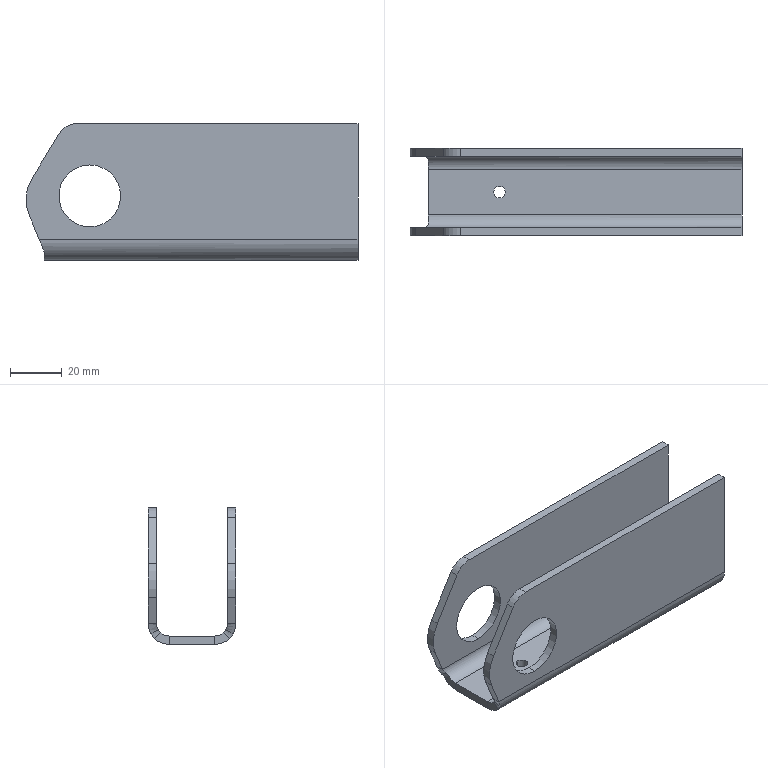Part | SolidWorks | features ICE 2, Fillet 1, FlatPattern 1, SMBaseFlange 1, SheetMetal 1 | 1 solid | 38 faces | box 128.757 x 34 x 53 mm | volume 47449 mm3 | plane 20 | cylinder 14 | spline 4 | commonest cylinder face diameters 24 x4 4.5 x2 10 x2 16 x2 16.4 x2 30 x2
STEP:
#1=CARTESIAN_POINT('',(41.,-14.75,-49.8));
#2=VERTEX_POINT('',#1);
#3=CARTESIAN_POINT('',(41.,-19.25,-49.8));
#4=VERTEX_POINT('',#3);
#5=CARTESIAN_POINT('',(41.,-17.,-49.8));
#6=DIRECTION('',(0.,0.,1.));
#7=DIRECTION('',(0.,1.,0.));
#8=AXIS2_PLACEMENT_3D('',#5,#6,#7);
#9=CIRCLE('',#8,2.25);
#10=EDGE_CURVE('',#2,#4,#9,.T.);
#11=ORIENTED_EDGE('',*,*,#10,.T.);
#12=CARTESIAN_POINT('',(41.,-19.25,-53.));
#13=VERTEX_POINT('',#12);
#14=CARTESIAN_POINT('',(41.,-19.25,0.001));
#15=DIRECTION('',(0.,0.,-1.));
#16=VECTOR('',#15,1000.);
#17=LINE('',#14,#16);
#18=EDGE_CURVE('',#4,#13,#17,.T.);
#19=ORIENTED_EDGE('',*,*,#18,.T.);
#20=CARTESIAN_POINT('',(41.,-14.75,-53.));
#21=VERTEX_POINT('',#20);
#22=CARTESIAN_POINT('',(41.,-17.,-53.));
#23=DIRECTION('',(0.,0.,-1.));
#24=DIRECTION('',(0.,1.,0.));
#25=AXIS2_PLACEMENT_3D('',#22,#23,#24);
#26=CIRCLE('',#25,2.25);
#27=EDGE_CURVE('',#13,#21,#26,.T.);
#28=ORIENTED_EDGE('',*,*,#27,.T.);
#29=CARTESIAN_POINT('',(41.,-14.75,0.001));
#30=DIRECTION('',(0.,0.,-1.));
#31=VECTOR('',#30,1000.);
#32=LINE('',#29,#31);
#33=EDGE_CURVE('',#2,#21,#32,.T.);
#34=ORIENTED_EDGE('',*,*,#33,.F.);
#35=EDGE_LOOP('',(#11,#19,#28,#34));
#36=FACE_OUTER_BOUND('',#35,.T.);
#37=CARTESIAN_POINT('',(41.,-17.,0.001));
#38=DIRECTION('',(0.,0.,-1.));
#39=DIRECTION('',(0.,1.,0.));
#40=AXIS2_PLACEMENT_3D('',#37,#38,#39);
#41=CYLINDRICAL_SURFACE('',#40,2.25);
#42=ADVANCED_FACE('',(#36),#41,.F.);
#43=CARTESIAN_POINT('',(31.,-30.8,-16.));
#44=VERTEX_POINT('',#43);
#45=CARTESIAN_POINT('',(31.,-30.8,-40.));
#46=VERTEX_POINT('',#45);
#47=CARTESIAN_POINT('',(31.,-30.8,-28.));
#48=DIRECTION('',(0.,-1.,0.));
#49=DIRECTION('',(0.,0.,1.));
#50=AXIS2_PLACEMENT_3D('',#47,#48,#49);
#51=CIRCLE('',#50,12.);
#52=EDGE_CURVE('',#44,#46,#51,.T.);
#53=ORIENTED_EDGE('',*,*,#52,.F.);
#54=CARTESIAN_POINT('',(31.,-34.,-16.));
#55=VERTEX_POINT('',#54);
#56=CARTESIAN_POINT('',(31.,-30.8,-16.));
#57=DIRECTION('',(0.,-1.,0.));
#58=VECTOR('',#57,1000.);
#59=LINE('',#56,#58);
#60=EDGE_CURVE('',#44,#55,#59,.T.);
#61=ORIENTED_EDGE('',*,*,#60,.T.);
#62=CARTESIAN_POINT('',(31.,-34.,-40.));
#63=VERTEX_POINT('',#62);
#64=CARTESIAN_POINT('',(31.,-34.,-28.));
#65=DIRECTION('',(0.,-1.,0.));
#66=DIRECTION('',(0.,0.,-1.));
#67=AXIS2_PLACEMENT_3D('',#64,#65,#66);
#68=CIRCLE('',#67,12.);
#69=EDGE_CURVE('',#55,#63,#68,.T.);
#70=ORIENTED_EDGE('',*,*,#69,.T.);
#71=CARTESIAN_POINT('',(31.,-30.8,-40.));
#72=DIRECTION('',(0.,-1.,0.));
#73=VECTOR('',#72,1000.);
#74=LINE('',#71,#73);
#75=EDGE_CURVE('',#46,#63,#74,.T.);
#76=ORIENTED_EDGE('',*,*,#75,.F.);
#77=EDGE_LOOP('',(#53,#61,#70,#76));
#78=FACE_OUTER_BOUND('',#77,.T.);
#79=CARTESIAN_POINT('',(31.,-30.8,-28.));
#80=DIRECTION('',(0.,-1.,0.));
#81=DIRECTION('',(0.,0.,-1.));
#82=AXIS2_PLACEMENT_3D('',#79,#80,#81);
#83=CYLINDRICAL_SURFACE('',#82,12.);
#84=ADVANCED_FACE('',(#78),#83,.F.);
#85=CARTESIAN_POINT('',(31.,-3.2,-40.));
#86=VERTEX_POINT('',#85);
#87=CARTESIAN_POINT('',(31.,-3.2,-16.));
#88=VERTEX_POINT('',#87);
#89=CARTESIAN_POINT('',(31.,-3.2,-28.));
#90=DIRECTION('',(0.,1.,0.));
#91=DIRECTION('',(0.,0.,-1.));
#92=AXIS2_PLACEMENT_3D('',#89,#90,#91);
#93=CIRCLE('',#92,12.);
#94=EDGE_CURVE('',#86,#88,#93,.T.);
#95=ORIENTED_EDGE('',*,*,#94,.F.);
#96=CARTESIAN_POINT('',(31.,0.,-40.));
#97=VERTEX_POINT('',#96);
#98=CARTESIAN_POINT('',(31.,-3.2,-40.));
#99=DIRECTION('',(0.,1.,0.));
#100=VECTOR('',#99,1000.);
#101=LINE('',#98,#100);
#102=EDGE_CURVE('',#86,#97,#101,.T.);
#103=ORIENTED_EDGE('',*,*,#102,.T.);
#104=CARTESIAN_POINT('',(31.,0.,-16.));
#105=VERTEX_POINT('',#104);
#106=CARTESIAN_POINT('',(31.,0.,-28.));
#107=DIRECTION('',(0.,1.,0.));
#108=DIRECTION('',(0.,0.,1.));
#109=AXIS2_PLACEMENT_3D('',#106,#107,#108);
#110=CIRCLE('',#109,12.);
#111=EDGE_CURVE('',#97,#105,#110,.T.);
#112=ORIENTED_EDGE('',*,*,#111,.T.);
#113=CARTESIAN_POINT('',(31.,-3.2,-16.));
#114=DIRECTION('',(0.,1.,0.));
#115=VECTOR('',#114,1000.);
#116=LINE('',#113,#115);
#117=EDGE_CURVE('',#88,#105,#116,.T.);
#118=ORIENTED_EDGE('',*,*,#117,.F.);
#119=EDGE_LOOP('',(#95,#103,#112,#118));
#120=FACE_OUTER_BOUND('',#119,.T.);
#121=CARTESIAN_POINT('',(31.,-3.2,-28.));
#122=DIRECTION('',(0.,1.,0.));
#123=DIRECTION('',(0.,0.,1.));
#124=AXIS2_PLACEMENT_3D('',#121,#122,#123);
#125=CYLINDRICAL_SURFACE('',#124,12.);
#126=ADVANCED_FACE('',(#120),#125,.F.);
#127=CARTESIAN_POINT('',(135.,-30.8,0.));
#128=VERTEX_POINT('',#127);
#129=CARTESIAN_POINT('',(26.002,-30.8,0.));
#130=VERTEX_POINT('',#129);
#131=CARTESIAN_POINT('',(135.,-30.8,0.));
#132=DIRECTION('',(-1.,0.,0.));
#133=VECTOR('',#132,1000.);
#134=LINE('',#131,#133);
#135=EDGE_CURVE('',#128,#130,#134,.T.);
#136=ORIENTED_EDGE('',*,*,#135,.T.);
#137=CARTESIAN_POINT('',(26.002,-34.,0.));
#138=VERTEX_POINT('',#137);
#139=CARTESIAN_POINT('',(26.002,-34.,0.));
#140=DIRECTION('',(0.,-1.,0.));
#141=VECTOR('',#140,1000.);
#142=LINE('',#139,#141);
#143=EDGE_CURVE('',#130,#138,#142,.T.);
#144=ORIENTED_EDGE('',*,*,#143,.T.);
#145=CARTESIAN_POINT('',(135.,-34.,0.));
#146=VERTEX_POINT('',#145);
#147=CARTESIAN_POINT('',(135.,-34.,0.));
#148=DIRECTION('',(-1.,0.,0.));
#149=VECTOR('',#148,1000.);
#150=LINE('',#147,#149);
#151=EDGE_CURVE('',#146,#138,#150,.T.);
#152=ORIENTED_EDGE('',*,*,#151,.F.);
#153=CARTESIAN_POINT('',(135.,-34.,0.));
#154=DIRECTION('',(0.,1.,0.));
#155=VECTOR('',#154,1000.);
#156=LINE('',#153,#155);
#157=EDGE_CURVE('',#146,#128,#156,.T.);
#158=ORIENTED_EDGE('',*,*,#157,.T.);
#159=EDGE_LOOP('',(#136,#144,#152,#158));
#160=FACE_OUTER_BOUND('',#159,.T.);
#161=CARTESIAN_POINT('',(135.,-34.,0.));
#162=DIRECTION('',(0.,0.,1.));
#163=DIRECTION('',(1.,0.,0.));
#164=AXIS2_PLACEMENT_3D('',#161,#162,#163);
#165=PLANE('',#164);
#166=ADVANCED_FACE('',(#160),#165,.T.);
#167=CARTESIAN_POINT('',(13.4,-31.409,-50.781));
#168=VERTEX_POINT('',#167);
#169=CARTESIAN_POINT('',(13.029,-32.906,-48.891));
#170=VERTEX_POINT('',#169);
#171=CARTESIAN_POINT('',(13.4,-31.409,-50.781));
#172=CARTESIAN_POINT('',(13.4,-31.709,-50.5));
#173=CARTESIAN_POINT('',(13.376,-31.987,-50.197));
#174=CARTESIAN_POINT('',(13.259,-32.491,-49.558));
#175=CARTESIAN_POINT('',(13.166,-32.713,-49.228));
#176=CARTESIAN_POINT('',(13.029,-32.906,-48.891));
#177=B_SPLINE_CURVE_WITH_KNOTS('',3,(#171,#172,#173,#174,#175,#176),.UNSPECIFIED.,.F.,.F.,(4,2,4),(0.,0.001232,0.002463),.UNSPECIFIED.);
#178=EDGE_CURVE('',#168,#170,#177,.T.);
#179=ORIENTED_EDGE('',*,*,#178,.F.);
#180=CARTESIAN_POINT('',(13.4,-25.8,-53.));
#181=VERTEX_POINT('',#180);
#182=CARTESIAN_POINT('',(13.4,-25.8,-44.8));
#183=DIRECTION('',(1.,0.,0.));
#184=DIRECTION('',(0.,0.,-1.));
#185=AXIS2_PLACEMENT_3D('',#182,#183,#184);
#186=CIRCLE('',#185,8.2);
#187=EDGE_CURVE('',#168,#181,#186,.T.);
#188=ORIENTED_EDGE('',*,*,#187,.T.);
#189=CARTESIAN_POINT('',(135.,-25.8,-53.));
#190=VERTEX_POINT('',#189);
#191=CARTESIAN_POINT('',(135.,-25.8,-53.));
#192=DIRECTION('',(-1.,0.,0.));
#193=VECTOR('',#192,1000.);
#194=LINE('',#191,#193);
#195=EDGE_CURVE('',#190,#181,#194,.T.);
#196=ORIENTED_EDGE('',*,*,#195,.F.);
#197=CARTESIAN_POINT('',(135.,-34.,-44.8));
#198=VERTEX_POINT('',#197);
#199=CARTESIAN_POINT('',(135.,-25.8,-44.8));
#200=DIRECTION('',(-1.,0.,0.));
#201=DIRECTION('',(0.,0.,-1.));
#202=AXIS2_PLACEMENT_3D('',#199,#200,#201);
#203=CIRCLE('',#202,8.2);
#204=EDGE_CURVE('',#190,#198,#203,.T.);
#205=ORIENTED_EDGE('',*,*,#204,.T.);
#206=CARTESIAN_POINT('',(11.359,-34.,-44.8));
#207=VERTEX_POINT('',#206);
#208=CARTESIAN_POINT('',(135.,-34.,-44.8));
#209=DIRECTION('',(-1.,0.,0.));
#210=VECTOR('',#209,1000.);
#211=LINE('',#208,#210);
#212=EDGE_CURVE('',#198,#207,#211,.T.);
#213=ORIENTED_EDGE('',*,*,#212,.T.);
#214=CARTESIAN_POINT('',(13.029,-32.906,-48.891));
#215=CARTESIAN_POINT('',(12.518,-33.627,-47.64));
#216=CARTESIAN_POINT('',(11.948,-34.,-46.244));
#217=CARTESIAN_POINT('',(11.359,-34.,-44.8));
#218=(BOUNDED_CURVE()B_SPLINE_CURVE(3,(#214,#215,#216,#217),.UNSPECIFIED.,.F.,.F.)B_SPLINE_CURVE_WITH_KNOTS((4,4),(4.19,4.712),.UNSPECIFIED.)CURVE()GEOMETRIC_REPRESENTATION_ITEM()RATIONAL_B_SPLINE_CURVE((1.,0.9774,0.9774,1.))REPRESENTATION_ITEM(''));
#219=EDGE_CURVE('',#170,#207,#218,.T.);
#220=ORIENTED_EDGE('',*,*,#219,.F.);
#221=EDGE_LOOP('',(#179,#188,#196,#205,#213,#220));
#222=FACE_OUTER_BOUND('',#221,.T.);
#223=CARTESIAN_POINT('',(135.,-25.8,-44.8));
#224=DIRECTION('',(-1.,0.,0.));
#225=DIRECTION('',(0.,0.,1.));
#226=AXIS2_PLACEMENT_3D('',#223,#224,#225);
#227=CYLINDRICAL_SURFACE('',#226,8.2);
#228=ADVANCED_FACE('',(#222),#227,.T.);
#229=CARTESIAN_POINT('',(41.,-17.,-53.));
#230=DIRECTION('',(0.,0.,-1.));
#231=DIRECTION('',(0.,1.,0.));
#232=AXIS2_PLACEMENT_3D('',#229,#230,#231);
#233=CIRCLE('',#232,2.25);
#234=EDGE_CURVE('',#21,#13,#233,.T.);
#235=ORIENTED_EDGE('',*,*,#234,.F.);
#236=ORIENTED_EDGE('',*,*,#27,.F.);
#237=EDGE_LOOP('',(#235,#236));
#238=FACE_BOUND('',#237,.T.);
#239=ORIENTED_EDGE('',*,*,#195,.T.);
#240=CARTESIAN_POINT('',(13.4,-8.2,-53.));
#241=VERTEX_POINT('',#240);
#242=CARTESIAN_POINT('',(13.4,-34.,-53.));
#243=DIRECTION('',(0.,1.,0.));
#244=VECTOR('',#243,1000.);
#245=LINE('',#242,#244);
#246=EDGE_CURVE('',#181,#241,#245,.T.);
#247=ORIENTED_EDGE('',*,*,#246,.T.);
#248=CARTESIAN_POINT('',(135.,-8.2,-53.));
#249=VERTEX_POINT('',#248);
#250=CARTESIAN_POINT('',(135.,-8.2,-53.));
#251=DIRECTION('',(-1.,0.,0.));
#252=VECTOR('',#251,1000.);
#253=LINE('',#250,#252);
#254=EDGE_CURVE('',#249,#241,#253,.T.);
#255=ORIENTED_EDGE('',*,*,#254,.F.);
#256=CARTESIAN_POINT('',(135.,0.,-53.));
#257=DIRECTION('',(0.,-1.,0.));
#258=VECTOR('',#257,1000.);
#259=LINE('',#256,#258);
#260=EDGE_CURVE('',#249,#190,#259,.T.);
#261=ORIENTED_EDGE('',*,*,#260,.T.);
#262=EDGE_LOOP('',(#239,#247,#255,#261));
#263=FACE_OUTER_BOUND('',#262,.T.);
#264=CARTESIAN_POINT('',(135.,0.,-53.));
#265=DIRECTION('',(0.,0.,-1.));
#266=DIRECTION('',(0.,1.,0.));
#267=AXIS2_PLACEMENT_3D('',#264,#265,#266);
#268=PLANE('',#267);
#269=ADVANCED_FACE('',(#238,#263),#268,.T.);
#270=ORIENTED_EDGE('',*,*,#254,.T.);
#271=CARTESIAN_POINT('',(13.4,-2.591,-50.781));
#272=VERTEX_POINT('',#271);
#273=CARTESIAN_POINT('',(13.4,-8.2,-44.8));
#274=DIRECTION('',(1.,0.,0.));
#275=DIRECTION('',(0.,0.,-1.));
#276=AXIS2_PLACEMENT_3D('',#273,#274,#275);
#277=CIRCLE('',#276,8.2);
#278=EDGE_CURVE('',#241,#272,#277,.T.);
#279=ORIENTED_EDGE('',*,*,#278,.T.);
#280=CARTESIAN_POINT('',(13.029,-1.094,-48.891));
#281=VERTEX_POINT('',#280);
#282=CARTESIAN_POINT('',(13.029,-1.094,-48.891));
#283=CARTESIAN_POINT('',(13.166,-1.287,-49.227));
#284=CARTESIAN_POINT('',(13.26,-1.511,-49.561));
#285=CARTESIAN_POINT('',(13.377,-2.015,-50.199));
#286=CARTESIAN_POINT('',(13.4,-2.291,-50.5));
#287=CARTESIAN_POINT('',(13.4,-2.591,-50.781));
#288=B_SPLINE_CURVE_WITH_KNOTS('',3,(#282,#283,#284,#285,#286,#287),.UNSPECIFIED.,.F.,.F.,(4,2,4),(0.,0.001231,0.002461),.UNSPECIFIED.);
#289=EDGE_CURVE('',#281,#272,#288,.T.);
#290=ORIENTED_EDGE('',*,*,#289,.F.);
#291=CARTESIAN_POINT('',(11.359,0.,-44.8));
#292=VERTEX_POINT('',#291);
#293=CARTESIAN_POINT('',(11.359,0.,-44.8));
#294=CARTESIAN_POINT('',(11.948,0.,-46.244));
#295=CARTESIAN_POINT('',(12.518,-0.373,-47.64));
#296=CARTESIAN_POINT('',(13.029,-1.094,-48.891));
#297=(BOUNDED_CURVE()B_SPLINE_CURVE(3,(#293,#294,#295,#296),.UNSPECIFIED.,.F.,.F.)B_SPLINE_CURVE_WITH_KNOTS((4,4),(1.571,2.093),.UNSPECIFIED.)CURVE()GEOMETRIC_REPRESENTATION_ITEM()RATIONAL_B_SPLINE_CURVE((1.,0.9774,0.9774,1.))REPRESENTATION_ITEM(''));
#298=EDGE_CURVE('',#292,#281,#297,.T.);
#299=ORIENTED_EDGE('',*,*,#298,.F.);
#300=CARTESIAN_POINT('',(135.,0.,-44.8));
#301=VERTEX_POINT('',#300);
#302=CARTESIAN_POINT('',(135.,0.,-44.8));
#303=DIRECTION('',(-1.,0.,0.));
#304=VECTOR('',#303,1000.);
#305=LINE('',#302,#304);
#306=EDGE_CURVE('',#301,#292,#305,.T.);
#307=ORIENTED_EDGE('',*,*,#306,.F.);
#308=CARTESIAN_POINT('',(135.,-8.2,-44.8));
#309=DIRECTION('',(-1.,0.,0.));
#310=DIRECTION('',(0.,0.,-1.));
#311=AXIS2_PLACEMENT_3D('',#308,#309,#310);
#312=CIRCLE('',#311,8.2);
#313=EDGE_CURVE('',#301,#249,#312,.T.);
#314=ORIENTED_EDGE('',*,*,#313,.T.);
#315=EDGE_LOOP('',(#270,#279,#290,#299,#307,#314));
#316=FACE_OUTER_BOUND('',#315,.T.);
#317=CARTESIAN_POINT('',(135.,-8.2,-44.8));
#318=DIRECTION('',(-1.,0.,0.));
#319=DIRECTION('',(0.,0.,1.));
#320=AXIS2_PLACEMENT_3D('',#317,#318,#319);
#321=CYLINDRICAL_SURFACE('',#320,8.2);
#322=ADVANCED_FACE('',(#316),#321,.T.);
#323=CARTESIAN_POINT('',(19.164,0.,-3.848));
#324=VERTEX_POINT('',#323);
#325=CARTESIAN_POINT('',(8.421,0.,-21.541));
#326=VERTEX_POINT('',#325);
#327=CARTESIAN_POINT('',(21.5,0.,0.));
#328=DIRECTION('',(-0.519,0.,-0.8548));
#329=VECTOR('',#328,1000.);
#330=LINE('',#327,#329);
#331=EDGE_CURVE('',#324,#326,#330,.T.);
#332=ORIENTED_EDGE('',*,*,#331,.F.);
#333=CARTESIAN_POINT('',(26.002,0.,0.));
#334=VERTEX_POINT('',#333);
#335=CARTESIAN_POINT('',(26.002,0.,-8.));
#336=DIRECTION('',(0.,1.,0.));
#337=DIRECTION('',(0.,0.,1.));
#338=AXIS2_PLACEMENT_3D('',#335,#336,#337);
#339=CIRCLE('',#338,8.);
#340=EDGE_CURVE('',#324,#334,#339,.T.);
#341=ORIENTED_EDGE('',*,*,#340,.T.);
#342=CARTESIAN_POINT('',(135.,0.,0.));
#343=VERTEX_POINT('',#342);
#344=CARTESIAN_POINT('',(135.,0.,0.));
#345=DIRECTION('',(-1.,0.,0.));
#346=VECTOR('',#345,1000.);
#347=LINE('',#344,#346);
#348=EDGE_CURVE('',#343,#334,#347,.T.);
#349=ORIENTED_EDGE('',*,*,#348,.F.);
#350=CARTESIAN_POINT('',(135.,0.,0.));
#351=DIRECTION('',(0.,0.,-1.));
#352=VECTOR('',#351,1000.);
#353=LINE('',#350,#352);
#354=EDGE_CURVE('',#343,#301,#353,.T.);
#355=ORIENTED_EDGE('',*,*,#354,.T.);
#356=ORIENTED_EDGE('',*,*,#306,.T.);
#357=CARTESIAN_POINT('',(7.356,0.,-34.995));
#358=VERTEX_POINT('',#357);
#359=CARTESIAN_POINT('',(7.356,0.,-34.995));
#360=DIRECTION('',(0.378,0.,-0.9258));
#361=VECTOR('',#360,1000.);
#362=LINE('',#359,#361);
#363=EDGE_CURVE('',#358,#292,#362,.T.);
#364=ORIENTED_EDGE('',*,*,#363,.F.);
#365=CARTESIAN_POINT('',(21.243,0.,-29.326));
#366=DIRECTION('',(0.,-1.,0.));
#367=DIRECTION('',(0.,0.,-1.));
#368=AXIS2_PLACEMENT_3D('',#365,#366,#367);
#369=CIRCLE('',#368,15.);
#370=EDGE_CURVE('',#326,#358,#369,.T.);
#371=ORIENTED_EDGE('',*,*,#370,.F.);
#372=EDGE_LOOP('',(#332,#341,#349,#355,#356,#364,#371));
#373=FACE_OUTER_BOUND('',#372,.T.);
#374=CARTESIAN_POINT('',(31.,0.,-28.));
#375=DIRECTION('',(0.,1.,0.));
#376=DIRECTION('',(0.,0.,1.));
#377=AXIS2_PLACEMENT_3D('',#374,#375,#376);
#378=CIRCLE('',#377,12.);
#379=EDGE_CURVE('',#105,#97,#378,.T.);
#380=ORIENTED_EDGE('',*,*,#379,.F.);
#381=ORIENTED_EDGE('',*,*,#111,.F.);
#382=EDGE_LOOP('',(#380,#381));
#383=FACE_BOUND('',#382,.T.);
#384=CARTESIAN_POINT('',(135.,0.,0.));
#385=DIRECTION('',(0.,1.,0.));
#386=DIRECTION('',(0.,0.,1.));
#387=AXIS2_PLACEMENT_3D('',#384,#385,#386);
#388=PLANE('',#387);
#389=ADVANCED_FACE('',(#373,#383),#388,.T.);
#390=ORIENTED_EDGE('',*,*,#348,.T.);
#391=CARTESIAN_POINT('',(26.002,-3.2,0.));
#392=VERTEX_POINT('',#391);
#393=CARTESIAN_POINT('',(26.002,-3.2,0.));
#394=DIRECTION('',(0.,-1.,0.));
#395=VECTOR('',#394,1000.);
#396=LINE('',#393,#395);
#397=EDGE_CURVE('',#334,#392,#396,.T.);
#398=ORIENTED_EDGE('',*,*,#397,.T.);
#399=CARTESIAN_POINT('',(135.,-3.2,0.));
#400=VERTEX_POINT('',#399);
#401=CARTESIAN_POINT('',(135.,-3.2,0.));
#402=DIRECTION('',(-1.,0.,0.));
#403=VECTOR('',#402,1000.);
#404=LINE('',#401,#403);
#405=EDGE_CURVE('',#400,#392,#404,.T.);
#406=ORIENTED_EDGE('',*,*,#405,.F.);
#407=CARTESIAN_POINT('',(135.,-3.2,0.));
#408=DIRECTION('',(0.,1.,0.));
#409=VECTOR('',#408,1000.);
#410=LINE('',#407,#409);
#411=EDGE_CURVE('',#400,#343,#410,.T.);
#412=ORIENTED_EDGE('',*,*,#411,.T.);
#413=EDGE_LOOP('',(#390,#398,#406,#412));
#414=FACE_OUTER_BOUND('',#413,.T.);
#415=CARTESIAN_POINT('',(135.,-3.2,0.));
#416=DIRECTION('',(0.,0.,1.));
#417=DIRECTION('',(1.,0.,0.));
#418=AXIS2_PLACEMENT_3D('',#415,#416,#417);
#419=PLANE('',#418);
#420=ADVANCED_FACE('',(#414),#419,.T.);
#421=ORIENTED_EDGE('',*,*,#405,.T.);
#422=CARTESIAN_POINT('',(19.164,-3.2,-3.848));
#423=VERTEX_POINT('',#422);
#424=CARTESIAN_POINT('',(26.002,-3.2,-8.));
#425=DIRECTION('',(0.,-1.,0.));
#426=DIRECTION('',(0.,0.,1.));
#427=AXIS2_PLACEMENT_3D('',#424,#425,#426);
#428=CIRCLE('',#427,8.);
#429=EDGE_CURVE('',#392,#423,#428,.T.);
#430=ORIENTED_EDGE('',*,*,#429,.T.);
#431=CARTESIAN_POINT('',(8.421,-3.2,-21.541));
#432=VERTEX_POINT('',#431);
#433=CARTESIAN_POINT('',(21.5,-3.2,0.));
#434=DIRECTION('',(-0.519,0.,-0.8548));
#435=VECTOR('',#434,1000.);
#436=LINE('',#433,#435);
#437=EDGE_CURVE('',#423,#432,#436,.T.);
#438=ORIENTED_EDGE('',*,*,#437,.T.);
#439=CARTESIAN_POINT('',(7.356,-3.2,-34.995));
#440=VERTEX_POINT('',#439);
#441=CARTESIAN_POINT('',(21.243,-3.2,-29.326));
#442=DIRECTION('',(0.,-1.,0.));
#443=DIRECTION('',(0.,0.,-1.));
#444=AXIS2_PLACEMENT_3D('',#441,#442,#443);
#445=CIRCLE('',#444,15.);
#446=EDGE_CURVE('',#432,#440,#445,.T.);
#447=ORIENTED_EDGE('',*,*,#446,.T.);
#448=CARTESIAN_POINT('',(11.359,-3.2,-44.8));
#449=VERTEX_POINT('',#448);
#450=CARTESIAN_POINT('',(7.356,-3.2,-34.995));
#451=DIRECTION('',(0.378,0.,-0.9258));
#452=VECTOR('',#451,1000.);
#453=LINE('',#450,#452);
#454=EDGE_CURVE('',#440,#449,#453,.T.);
#455=ORIENTED_EDGE('',*,*,#454,.T.);
#456=CARTESIAN_POINT('',(135.,-3.2,-44.8));
#457=VERTEX_POINT('',#456);
#458=CARTESIAN_POINT('',(135.,-3.2,-44.8));
#459=DIRECTION('',(-1.,0.,0.));
#460=VECTOR('',#459,1000.);
#461=LINE('',#458,#460);
#462=EDGE_CURVE('',#457,#449,#461,.T.);
#463=ORIENTED_EDGE('',*,*,#462,.F.);
#464=CARTESIAN_POINT('',(135.,-3.2,0.));
#465=DIRECTION('',(0.,0.,-1.));
#466=VECTOR('',#465,1000.);
#467=LINE('',#464,#466);
#468=EDGE_CURVE('',#400,#457,#467,.T.);
#469=ORIENTED_EDGE('',*,*,#468,.F.);
#470=EDGE_LOOP('',(#421,#430,#438,#447,#455,#463,#469));
#471=FACE_OUTER_BOUND('',#470,.T.);
#472=CARTESIAN_POINT('',(31.,-3.2,-28.));
#473=DIRECTION('',(0.,1.,0.));
#474=DIRECTION('',(0.,0.,-1.));
#475=AXIS2_PLACEMENT_3D('',#472,#473,#474);
#476=CIRCLE('',#475,12.);
#477=EDGE_CURVE('',#88,#86,#476,.T.);
#478=ORIENTED_EDGE('',*,*,#477,.T.);
#479=ORIENTED_EDGE('',*,*,#94,.T.);
#480=EDGE_LOOP('',(#478,#479));
#481=FACE_BOUND('',#480,.T.);
#482=CARTESIAN_POINT('',(135.,-3.2,0.));
#483=DIRECTION('',(0.,1.,0.));
#484=DIRECTION('',(0.,0.,1.));
#485=AXIS2_PLACEMENT_3D('',#482,#483,#484);
#486=PLANE('',#485);
#487=ADVANCED_FACE('',(#471,#481),#486,.F.);
#488=CARTESIAN_POINT('',(13.4,-8.2,-49.8));
#489=VERTEX_POINT('',#488);
#490=CARTESIAN_POINT('',(13.4,-4.78,-48.447));
#491=VERTEX_POINT('',#490);
#492=CARTESIAN_POINT('',(13.4,-8.2,-44.8));
#493=DIRECTION('',(1.,0.,0.));
#494=DIRECTION('',(0.,0.,1.));
#495=AXIS2_PLACEMENT_3D('',#492,#493,#494);
#496=CIRCLE('',#495,5.);
#497=EDGE_CURVE('',#489,#491,#496,.T.);
#498=ORIENTED_EDGE('',*,*,#497,.F.);
#499=CARTESIAN_POINT('',(135.,-8.2,-49.8));
#500=VERTEX_POINT('',#499);
#501=CARTESIAN_POINT('',(135.,-8.2,-49.8));
#502=DIRECTION('',(-1.,0.,0.));
#503=VECTOR('',#502,1000.);
#504=LINE('',#501,#503);
#505=EDGE_CURVE('',#500,#489,#504,.T.);
#506=ORIENTED_EDGE('',*,*,#505,.F.);
#507=CARTESIAN_POINT('',(135.,-8.2,-44.8));
#508=DIRECTION('',(-1.,0.,0.));
#509=DIRECTION('',(0.,0.,-1.));
#510=AXIS2_PLACEMENT_3D('',#507,#508,#509);
#511=CIRCLE('',#510,5.);
#512=EDGE_CURVE('',#457,#500,#511,.T.);
#513=ORIENTED_EDGE('',*,*,#512,.F.);
#514=ORIENTED_EDGE('',*,*,#462,.T.);
#515=CARTESIAN_POINT('',(13.029,-3.867,-47.295));
#516=VERTEX_POINT('',#515);
#517=CARTESIAN_POINT('',(11.359,-3.2,-44.8));
#518=CARTESIAN_POINT('',(11.948,-3.2,-45.681));
#519=CARTESIAN_POINT('',(12.518,-3.427,-46.532));
#520=CARTESIAN_POINT('',(13.029,-3.867,-47.295));
#521=(BOUNDED_CURVE()B_SPLINE_CURVE(3,(#517,#518,#519,#520),.UNSPECIFIED.,.F.,.F.)B_SPLINE_CURVE_WITH_KNOTS((4,4),(1.571,2.093),.UNSPECIFIED.)CURVE()GEOMETRIC_REPRESENTATION_ITEM()RATIONAL_B_SPLINE_CURVE((1.,0.9774,0.9774,1.))REPRESENTATION_ITEM(''));
#522=EDGE_CURVE('',#449,#516,#521,.T.);
#523=ORIENTED_EDGE('',*,*,#522,.T.);
#524=CARTESIAN_POINT('',(13.029,-3.867,-47.295));
#525=CARTESIAN_POINT('',(13.158,-3.978,-47.488));
#526=CARTESIAN_POINT('',(13.253,-4.111,-47.688));
#527=CARTESIAN_POINT('',(13.375,-4.418,-48.08));
#528=CARTESIAN_POINT('',(13.4,-4.592,-48.271));
#529=CARTESIAN_POINT('',(13.4,-4.78,-48.447));
#530=B_SPLINE_CURVE_WITH_KNOTS('',3,(#524,#525,#526,#527,#528,#529),.UNSPECIFIED.,.F.,.F.,(4,2,4),(0.,0.0007664,0.001533),.UNSPECIFIED.);
#531=EDGE_CURVE('',#516,#491,#530,.T.);
#532=ORIENTED_EDGE('',*,*,#531,.T.);
#533=EDGE_LOOP('',(#498,#506,#513,#514,#523,#532));
#534=FACE_OUTER_BOUND('',#533,.T.);
#535=CARTESIAN_POINT('',(135.,-8.2,-44.8));
#536=DIRECTION('',(-1.,0.,0.));
#537=DIRECTION('',(0.,0.,1.));
#538=AXIS2_PLACEMENT_3D('',#535,#536,#537);
#539=CYLINDRICAL_SURFACE('',#538,5.);
#540=ADVANCED_FACE('',(#534),#539,.F.);
#541=ORIENTED_EDGE('',*,*,#10,.F.);
#542=CARTESIAN_POINT('',(41.,-17.,-49.8));
#543=DIRECTION('',(0.,0.,1.));
#544=DIRECTION('',(0.,1.,0.));
#545=AXIS2_PLACEMENT_3D('',#542,#543,#544);
#546=CIRCLE('',#545,2.25);
#547=EDGE_CURVE('',#4,#2,#546,.T.);
#548=ORIENTED_EDGE('',*,*,#547,.F.);
#549=EDGE_LOOP('',(#541,#548));
#550=FACE_BOUND('',#549,.T.);
#551=CARTESIAN_POINT('',(13.4,-25.8,-49.8));
#552=VERTEX_POINT('',#551);
#553=CARTESIAN_POINT('',(13.4,0.,-49.8));
#554=DIRECTION('',(0.,1.,0.));
#555=VECTOR('',#554,1000.);
#556=LINE('',#553,#555);
#557=EDGE_CURVE('',#552,#489,#556,.T.);
#558=ORIENTED_EDGE('',*,*,#557,.F.);
#559=CARTESIAN_POINT('',(135.,-25.8,-49.8));
#560=VERTEX_POINT('',#559);
#561=CARTESIAN_POINT('',(135.,-25.8,-49.8));
#562=DIRECTION('',(-1.,0.,0.));
#563=VECTOR('',#562,1000.);
#564=LINE('',#561,#563);
#565=EDGE_CURVE('',#560,#552,#564,.T.);
#566=ORIENTED_EDGE('',*,*,#565,.F.);
#567=CARTESIAN_POINT('',(135.,0.,-49.8));
#568=DIRECTION('',(0.,-1.,0.));
#569=VECTOR('',#568,1000.);
#570=LINE('',#567,#569);
#571=EDGE_CURVE('',#500,#560,#570,.T.);
#572=ORIENTED_EDGE('',*,*,#571,.F.);
#573=ORIENTED_EDGE('',*,*,#505,.T.);
#574=EDGE_LOOP('',(#558,#566,#572,#573));
#575=FACE_OUTER_BOUND('',#574,.T.);
#576=CARTESIAN_POINT('',(135.,0.,-49.8));
#577=DIRECTION('',(0.,0.,-1.));
#578=DIRECTION('',(0.,1.,0.));
#579=AXIS2_PLACEMENT_3D('',#576,#577,#578);
#580=PLANE('',#579);
#581=ADVANCED_FACE('',(#550,#575),#580,.F.);
#582=CARTESIAN_POINT('',(13.4,-29.22,-48.447));
#583=VERTEX_POINT('',#582);
#584=CARTESIAN_POINT('',(13.4,-25.8,-44.8));
#585=DIRECTION('',(1.,0.,0.));
#586=DIRECTION('',(0.,0.,1.));
#587=AXIS2_PLACEMENT_3D('',#584,#585,#586);
#588=CIRCLE('',#587,5.);
#589=EDGE_CURVE('',#583,#552,#588,.T.);
#590=ORIENTED_EDGE('',*,*,#589,.F.);
#591=CARTESIAN_POINT('',(13.029,-30.133,-47.295));
#592=VERTEX_POINT('',#591);
#593=CARTESIAN_POINT('',(13.4,-29.22,-48.447));
#594=CARTESIAN_POINT('',(13.4,-29.408,-48.271));
#595=CARTESIAN_POINT('',(13.375,-29.581,-48.081));
#596=CARTESIAN_POINT('',(13.254,-29.889,-47.689));
#597=CARTESIAN_POINT('',(13.158,-30.022,-47.488));
#598=CARTESIAN_POINT('',(13.029,-30.133,-47.295));
#599=B_SPLINE_CURVE_WITH_KNOTS('',3,(#593,#594,#595,#596,#597,#598),.UNSPECIFIED.,.F.,.F.,(4,2,4),(0.,0.0007674,0.001535),.UNSPECIFIED.);
#600=EDGE_CURVE('',#583,#592,#599,.T.);
#601=ORIENTED_EDGE('',*,*,#600,.T.);
#602=CARTESIAN_POINT('',(11.359,-30.8,-44.8));
#603=VERTEX_POINT('',#602);
#604=CARTESIAN_POINT('',(13.029,-30.133,-47.295));
#605=CARTESIAN_POINT('',(12.518,-30.573,-46.532));
#606=CARTESIAN_POINT('',(11.948,-30.8,-45.681));
#607=CARTESIAN_POINT('',(11.359,-30.8,-44.8));
#608=(BOUNDED_CURVE()B_SPLINE_CURVE(3,(#604,#605,#606,#607),.UNSPECIFIED.,.F.,.F.)B_SPLINE_CURVE_WITH_KNOTS((4,4),(4.19,4.712),.UNSPECIFIED.)CURVE()GEOMETRIC_REPRESENTATION_ITEM()RATIONAL_B_SPLINE_CURVE((1.,0.9774,0.9774,1.))REPRESENTATION_ITEM(''));
#609=EDGE_CURVE('',#592,#603,#608,.T.);
#610=ORIENTED_EDGE('',*,*,#609,.T.);
#611=CARTESIAN_POINT('',(135.,-30.8,-44.8));
#612=VERTEX_POINT('',#611);
#613=CARTESIAN_POINT('',(135.,-30.8,-44.8));
#614=DIRECTION('',(-1.,0.,0.));
#615=VECTOR('',#614,1000.);
#616=LINE('',#613,#615);
#617=EDGE_CURVE('',#612,#603,#616,.T.);
#618=ORIENTED_EDGE('',*,*,#617,.F.);
#619=CARTESIAN_POINT('',(135.,-25.8,-44.8));
#620=DIRECTION('',(-1.,0.,0.));
#621=DIRECTION('',(0.,0.,-1.));
#622=AXIS2_PLACEMENT_3D('',#619,#620,#621);
#623=CIRCLE('',#622,5.);
#624=EDGE_CURVE('',#560,#612,#623,.T.);
#625=ORIENTED_EDGE('',*,*,#624,.F.);
#626=ORIENTED_EDGE('',*,*,#565,.T.);
#627=EDGE_LOOP('',(#590,#601,#610,#618,#625,#626));
#628=FACE_OUTER_BOUND('',#627,.T.);
#629=CARTESIAN_POINT('',(135.,-25.8,-44.8));
#630=DIRECTION('',(-1.,0.,0.));
#631=DIRECTION('',(0.,0.,1.));
#632=AXIS2_PLACEMENT_3D('',#629,#630,#631);
#633=CYLINDRICAL_SURFACE('',#632,5.);
#634=ADVANCED_FACE('',(#628),#633,.F.);
#635=CARTESIAN_POINT('',(135.,-8.2,-53.));
#636=DIRECTION('',(0.,0.,1.));
#637=VECTOR('',#636,1000.);
#638=LINE('',#635,#637);
#639=EDGE_CURVE('',#249,#500,#638,.T.);
#640=ORIENTED_EDGE('',*,*,#639,.F.);
#641=ORIENTED_EDGE('',*,*,#313,.F.);
#642=CARTESIAN_POINT('',(135.,-3.2,-44.8));
#643=DIRECTION('',(0.,1.,0.));
#644=VECTOR('',#643,1000.);
#645=LINE('',#642,#644);
#646=EDGE_CURVE('',#457,#301,#645,.T.);
#647=ORIENTED_EDGE('',*,*,#646,.F.);
#648=ORIENTED_EDGE('',*,*,#512,.T.);
#649=EDGE_LOOP('',(#640,#641,#647,#648));
#650=FACE_OUTER_BOUND('',#649,.T.);
#651=CARTESIAN_POINT('',(135.,-8.2,-53.));
#652=DIRECTION('',(1.,0.,0.));
#653=DIRECTION('',(0.,0.,-1.));
#654=AXIS2_PLACEMENT_3D('',#651,#652,#653);
#655=PLANE('',#654);
#656=ADVANCED_FACE('',(#650),#655,.T.);
#657=ORIENTED_EDGE('',*,*,#260,.F.);
#658=ORIENTED_EDGE('',*,*,#639,.T.);
#659=ORIENTED_EDGE('',*,*,#571,.T.);
#660=CARTESIAN_POINT('',(135.,-25.8,-49.8));
#661=DIRECTION('',(0.,0.,-1.));
#662=VECTOR('',#661,1000.);
#663=LINE('',#660,#662);
#664=EDGE_CURVE('',#560,#190,#663,.T.);
#665=ORIENTED_EDGE('',*,*,#664,.T.);
#666=EDGE_LOOP('',(#657,#658,#659,#665));
#667=FACE_OUTER_BOUND('',#666,.T.);
#668=CARTESIAN_POINT('',(135.,-3.2,-44.8));
#669=DIRECTION('',(1.,0.,0.));
#670=DIRECTION('',(0.,0.,-1.));
#671=AXIS2_PLACEMENT_3D('',#668,#669,#670);
#672=PLANE('',#671);
#673=ADVANCED_FACE('',(#667),#672,.T.);
#674=CARTESIAN_POINT('',(135.,-34.,-44.8));
#675=DIRECTION('',(0.,1.,0.));
#676=VECTOR('',#675,1000.);
#677=LINE('',#674,#676);
#678=EDGE_CURVE('',#198,#612,#677,.T.);
#679=ORIENTED_EDGE('',*,*,#678,.F.);
#680=ORIENTED_EDGE('',*,*,#204,.F.);
#681=ORIENTED_EDGE('',*,*,#664,.F.);
#682=ORIENTED_EDGE('',*,*,#624,.T.);
#683=EDGE_LOOP('',(#679,#680,#681,#682));
#684=FACE_OUTER_BOUND('',#683,.T.);
#685=CARTESIAN_POINT('',(135.,-34.,-44.8));
#686=DIRECTION('',(1.,0.,0.));
#687=DIRECTION('',(0.,0.,-1.));
#688=AXIS2_PLACEMENT_3D('',#685,#686,#687);
#689=PLANE('',#688);
#690=ADVANCED_FACE('',(#684),#689,.T.);
#691=CARTESIAN_POINT('',(135.,-34.,-53.));
#692=DIRECTION('',(0.,0.,1.));
#693=VECTOR('',#692,1000.);
#694=LINE('',#691,#693);
#695=EDGE_CURVE('',#198,#146,#694,.T.);
#696=ORIENTED_EDGE('',*,*,#695,.F.);
#697=ORIENTED_EDGE('',*,*,#678,.T.);
#698=CARTESIAN_POINT('',(135.,-30.8,-53.));
#699=DIRECTION('',(0.,0.,1.));
#700=VECTOR('',#699,1000.);
#701=LINE('',#698,#700);
#702=EDGE_CURVE('',#612,#128,#701,.T.);
#703=ORIENTED_EDGE('',*,*,#702,.T.);
#704=ORIENTED_EDGE('',*,*,#157,.F.);
#705=EDGE_LOOP('',(#696,#697,#703,#704));
#706=FACE_OUTER_BOUND('',#705,.T.);
#707=CARTESIAN_POINT('',(135.,-25.8,-49.8));
#708=DIRECTION('',(1.,0.,0.));
#709=DIRECTION('',(0.,0.,-1.));
#710=AXIS2_PLACEMENT_3D('',#707,#708,#709);
#711=PLANE('',#710);
#712=ADVANCED_FACE('',(#706),#711,.T.);
#713=CARTESIAN_POINT('',(19.164,-30.8,-3.848));
#714=VERTEX_POINT('',#713);
#715=CARTESIAN_POINT('',(8.421,-30.8,-21.541));
#716=VERTEX_POINT('',#715);
#717=CARTESIAN_POINT('',(28.558,-30.8,11.625));
#718=DIRECTION('',(-0.519,0.,-0.8548));
#719=VECTOR('',#718,1000.);
#720=LINE('',#717,#719);
#721=EDGE_CURVE('',#714,#716,#720,.T.);
#722=ORIENTED_EDGE('',*,*,#721,.F.);
#723=CARTESIAN_POINT('',(26.002,-30.8,-8.));
#724=DIRECTION('',(0.,1.,0.));
#725=DIRECTION('',(0.,0.,-1.));
#726=AXIS2_PLACEMENT_3D('',#723,#724,#725);
#727=CIRCLE('',#726,8.);
#728=EDGE_CURVE('',#714,#130,#727,.T.);
#729=ORIENTED_EDGE('',*,*,#728,.T.);
#730=ORIENTED_EDGE('',*,*,#135,.F.);
#731=ORIENTED_EDGE('',*,*,#702,.F.);
#732=ORIENTED_EDGE('',*,*,#617,.T.);
#733=CARTESIAN_POINT('',(7.356,-30.8,-34.995));
#734=VERTEX_POINT('',#733);
#735=CARTESIAN_POINT('',(31.892,-30.8,-95.095));
#736=DIRECTION('',(0.378,0.,-0.9258));
#737=VECTOR('',#736,1000.);
#738=LINE('',#735,#737);
#739=EDGE_CURVE('',#734,#603,#738,.T.);
#740=ORIENTED_EDGE('',*,*,#739,.F.);
#741=CARTESIAN_POINT('',(21.243,-30.8,-29.326));
#742=DIRECTION('',(0.,-1.,0.));
#743=DIRECTION('',(0.,0.,-1.));
#744=AXIS2_PLACEMENT_3D('',#741,#742,#743);
#745=CIRCLE('',#744,15.);
#746=EDGE_CURVE('',#716,#734,#745,.T.);
#747=ORIENTED_EDGE('',*,*,#746,.F.);
#748=EDGE_LOOP('',(#722,#729,#730,#731,#732,#740,#747));
#749=FACE_OUTER_BOUND('',#748,.T.);
#750=CARTESIAN_POINT('',(31.,-30.8,-28.));
#751=DIRECTION('',(0.,-1.,0.));
#752=DIRECTION('',(0.,0.,1.));
#753=AXIS2_PLACEMENT_3D('',#750,#751,#752);
#754=CIRCLE('',#753,12.);
#755=EDGE_CURVE('',#46,#44,#754,.T.);
#756=ORIENTED_EDGE('',*,*,#755,.T.);
#757=ORIENTED_EDGE('',*,*,#52,.T.);
#758=EDGE_LOOP('',(#756,#757));
#759=FACE_BOUND('',#758,.T.);
#760=CARTESIAN_POINT('',(135.,-30.8,-53.));
#761=DIRECTION('',(0.,-1.,0.));
#762=DIRECTION('',(0.,0.,-1.));
#763=AXIS2_PLACEMENT_3D('',#760,#761,#762);
#764=PLANE('',#763);
#765=ADVANCED_FACE('',(#749,#759),#764,.F.);
#766=CARTESIAN_POINT('',(31.,-34.,-28.));
#767=DIRECTION('',(0.,-1.,0.));
#768=DIRECTION('',(0.,0.,-1.));
#769=AXIS2_PLACEMENT_3D('',#766,#767,#768);
#770=CIRCLE('',#769,12.);
#771=EDGE_CURVE('',#63,#55,#770,.T.);
#772=ORIENTED_EDGE('',*,*,#771,.F.);
#773=ORIENTED_EDGE('',*,*,#69,.F.);
#774=EDGE_LOOP('',(#772,#773));
#775=FACE_BOUND('',#774,.T.);
#776=ORIENTED_EDGE('',*,*,#151,.T.);
#777=CARTESIAN_POINT('',(19.164,-34.,-3.848));
#778=VERTEX_POINT('',#777);
#779=CARTESIAN_POINT('',(26.002,-34.,-8.));
#780=DIRECTION('',(0.,-1.,0.));
#781=DIRECTION('',(0.,0.,-1.));
#782=AXIS2_PLACEMENT_3D('',#779,#780,#781);
#783=CIRCLE('',#782,8.);
#784=EDGE_CURVE('',#138,#778,#783,.T.);
#785=ORIENTED_EDGE('',*,*,#784,.T.);
#786=CARTESIAN_POINT('',(8.421,-34.,-21.541));
#787=VERTEX_POINT('',#786);
#788=CARTESIAN_POINT('',(28.558,-34.,11.625));
#789=DIRECTION('',(-0.519,0.,-0.8548));
#790=VECTOR('',#789,1000.);
#791=LINE('',#788,#790);
#792=EDGE_CURVE('',#778,#787,#791,.T.);
#793=ORIENTED_EDGE('',*,*,#792,.T.);
#794=CARTESIAN_POINT('',(7.356,-34.,-34.995));
#795=VERTEX_POINT('',#794);
#796=CARTESIAN_POINT('',(21.243,-34.,-29.326));
#797=DIRECTION('',(0.,-1.,0.));
#798=DIRECTION('',(0.,0.,-1.));
#799=AXIS2_PLACEMENT_3D('',#796,#797,#798);
#800=CIRCLE('',#799,15.);
#801=EDGE_CURVE('',#787,#795,#800,.T.);
#802=ORIENTED_EDGE('',*,*,#801,.T.);
#803=CARTESIAN_POINT('',(31.892,-34.,-95.095));
#804=DIRECTION('',(0.378,0.,-0.9258));
#805=VECTOR('',#804,1000.);
#806=LINE('',#803,#805);
#807=EDGE_CURVE('',#795,#207,#806,.T.);
#808=ORIENTED_EDGE('',*,*,#807,.T.);
#809=ORIENTED_EDGE('',*,*,#212,.F.);
#810=ORIENTED_EDGE('',*,*,#695,.T.);
#811=EDGE_LOOP('',(#776,#785,#793,#802,#808,#809,#810));
#812=FACE_OUTER_BOUND('',#811,.T.);
#813=CARTESIAN_POINT('',(135.,-34.,-53.));
#814=DIRECTION('',(0.,-1.,0.));
#815=DIRECTION('',(0.,0.,-1.));
#816=AXIS2_PLACEMENT_3D('',#813,#814,#815);
#817=PLANE('',#816);
#818=ADVANCED_FACE('',(#775,#812),#817,.T.);
#819=ORIENTED_EDGE('',*,*,#468,.T.);
#820=ORIENTED_EDGE('',*,*,#646,.T.);
#821=ORIENTED_EDGE('',*,*,#354,.F.);
#822=ORIENTED_EDGE('',*,*,#411,.F.);
#823=EDGE_LOOP('',(#819,#820,#821,#822));
#824=FACE_OUTER_BOUND('',#823,.T.);
#825=CARTESIAN_POINT('',(135.,-25.8,-44.8));
#826=DIRECTION('',(1.,0.,0.));
#827=DIRECTION('',(0.,0.,-1.));
#828=AXIS2_PLACEMENT_3D('',#825,#826,#827);
#829=PLANE('',#828);
#830=ADVANCED_FACE('',(#824),#829,.T.);
#831=CARTESIAN_POINT('',(13.4,-31.409,-50.781));
#832=DIRECTION('',(0.,-0.6841,-0.7294));
#833=VECTOR('',#832,1000.);
#834=LINE('',#831,#833);
#835=EDGE_CURVE('',#583,#168,#834,.T.);
#836=ORIENTED_EDGE('',*,*,#835,.F.);
#837=ORIENTED_EDGE('',*,*,#589,.T.);
#838=CARTESIAN_POINT('',(13.4,-25.8,-53.));
#839=DIRECTION('',(0.,0.,1.));
#840=VECTOR('',#839,1000.);
#841=LINE('',#838,#840);
#842=EDGE_CURVE('',#181,#552,#841,.T.);
#843=ORIENTED_EDGE('',*,*,#842,.F.);
#844=ORIENTED_EDGE('',*,*,#187,.F.);
#845=EDGE_LOOP('',(#836,#837,#843,#844));
#846=FACE_OUTER_BOUND('',#845,.T.);
#847=CARTESIAN_POINT('',(13.4,-25.8,-44.8));
#848=DIRECTION('',(-1.,0.,0.));
#849=DIRECTION('',(0.,0.,1.));
#850=AXIS2_PLACEMENT_3D('',#847,#848,#849);
#851=PLANE('',#850);
#852=ADVANCED_FACE('',(#846),#851,.T.);
#853=ORIENTED_EDGE('',*,*,#835,.T.);
#854=ORIENTED_EDGE('',*,*,#178,.T.);
#855=CARTESIAN_POINT('',(13.029,-31.52,-48.093));
#856=DIRECTION('',(0.,0.8666,0.499));
#857=VECTOR('',#856,1000.);
#858=LINE('',#855,#857);
#859=EDGE_CURVE('',#170,#592,#858,.T.);
#860=ORIENTED_EDGE('',*,*,#859,.T.);
#861=ORIENTED_EDGE('',*,*,#600,.F.);
#862=EDGE_LOOP('',(#853,#854,#860,#861));
#863=FACE_OUTER_BOUND('',#862,.T.);
#864=CARTESIAN_POINT('',(13.4,-29.198,-48.424));
#865=CARTESIAN_POINT('',(13.4,-29.378,-48.256));
#866=CARTESIAN_POINT('',(13.376,-29.548,-48.07));
#867=CARTESIAN_POINT('',(13.259,-29.854,-47.683));
#868=CARTESIAN_POINT('',(13.166,-29.988,-47.482));
#869=CARTESIAN_POINT('',(13.029,-30.105,-47.279));
#870=CARTESIAN_POINT('',(13.4,-29.22,-48.447));
#871=CARTESIAN_POINT('',(13.4,-29.401,-48.278));
#872=CARTESIAN_POINT('',(13.376,-29.572,-48.091));
#873=CARTESIAN_POINT('',(13.259,-29.88,-47.701));
#874=CARTESIAN_POINT('',(13.166,-30.015,-47.5));
#875=CARTESIAN_POINT('',(13.029,-30.133,-47.295));
#876=CARTESIAN_POINT('',(13.4,-31.409,-50.781));
#877=CARTESIAN_POINT('',(13.4,-31.705,-50.504));
#878=CARTESIAN_POINT('',(13.376,-31.986,-50.198));
#879=CARTESIAN_POINT('',(13.259,-32.491,-49.558));
#880=CARTESIAN_POINT('',(13.166,-32.713,-49.228));
#881=CARTESIAN_POINT('',(13.029,-32.906,-48.891));
#882=CARTESIAN_POINT('',(13.4,-31.431,-50.805));
#883=CARTESIAN_POINT('',(13.4,-31.728,-50.526));
#884=CARTESIAN_POINT('',(13.376,-32.011,-50.219));
#885=CARTESIAN_POINT('',(13.259,-32.517,-49.577));
#886=CARTESIAN_POINT('',(13.166,-32.74,-49.245));
#887=CARTESIAN_POINT('',(13.029,-32.934,-48.908));
#888=B_SPLINE_SURFACE_WITH_KNOTS('',1,3,((#864,#865,#866,#867,#868,#869),(#870,#871,#872,#873,#874,#875),(#876,#877,#878,#879,#880,#881),(#882,#883,#884,#885,#886,#887)),.UNSPECIFIED.,.F.,.F.,.F.,(2,1,1,2),(4,2,4),(-0.01,0.,1.,1.01),(0.006172,0.007393,0.008614),.UNSPECIFIED.);
#889=ADVANCED_FACE('',(#863),#888,.T.);
#890=ORIENTED_EDGE('',*,*,#219,.T.);
#891=CARTESIAN_POINT('',(11.359,-34.,-44.8));
#892=DIRECTION('',(0.,1.,0.));
#893=VECTOR('',#892,1000.);
#894=LINE('',#891,#893);
#895=EDGE_CURVE('',#207,#603,#894,.T.);
#896=ORIENTED_EDGE('',*,*,#895,.T.);
#897=ORIENTED_EDGE('',*,*,#609,.F.);
#898=ORIENTED_EDGE('',*,*,#859,.F.);
#899=EDGE_LOOP('',(#890,#896,#897,#898));
#900=FACE_OUTER_BOUND('',#899,.T.);
#901=CARTESIAN_POINT('',(8.011,-25.8,-36.6));
#902=CARTESIAN_POINT('',(8.011,-25.8,-37.667));
#903=CARTESIAN_POINT('',(8.011,-25.8,-38.733));
#904=CARTESIAN_POINT('',(8.011,-25.8,-39.8));
#905=CARTESIAN_POINT('',(8.011,-9.4,-36.6));
#906=CARTESIAN_POINT('',(8.011,-11.533,-37.667));
#907=CARTESIAN_POINT('',(8.011,-13.667,-38.733));
#908=CARTESIAN_POINT('',(8.011,-15.8,-39.8));
#909=CARTESIAN_POINT('',(14.706,-9.4,-53.));
#910=CARTESIAN_POINT('',(14.706,-11.533,-51.933));
#911=CARTESIAN_POINT('',(14.706,-13.667,-50.867));
#912=CARTESIAN_POINT('',(14.706,-15.8,-49.8));
#913=CARTESIAN_POINT('',(14.706,-25.8,-53.));
#914=CARTESIAN_POINT('',(14.706,-25.8,-51.933));
#915=CARTESIAN_POINT('',(14.706,-25.8,-50.867));
#916=CARTESIAN_POINT('',(14.706,-25.8,-49.8));
#917=CARTESIAN_POINT('',(14.706,-42.2,-53.));
#918=CARTESIAN_POINT('',(14.706,-40.067,-51.933));
#919=CARTESIAN_POINT('',(14.706,-37.933,-50.867));
#920=CARTESIAN_POINT('',(14.706,-35.8,-49.8));
#921=CARTESIAN_POINT('',(8.011,-42.2,-36.6));
#922=CARTESIAN_POINT('',(8.011,-40.067,-37.667));
#923=CARTESIAN_POINT('',(8.011,-37.933,-38.733));
#924=CARTESIAN_POINT('',(8.011,-35.8,-39.8));
#925=CARTESIAN_POINT('',(8.011,-25.8,-36.6));
#926=CARTESIAN_POINT('',(8.011,-25.8,-37.667));
#927=CARTESIAN_POINT('',(8.011,-25.8,-38.733));
#928=CARTESIAN_POINT('',(8.011,-25.8,-39.8));
#929=(BOUNDED_SURFACE()B_SPLINE_SURFACE(3,3,((#901,#902,#903,#904),(#905,#906,#907,#908),(#909,#910,#911,#912),(#913,#914,#915,#916),(#917,#918,#919,#920),(#921,#922,#923,#924),(#925,#926,#927,#928)),.UNSPECIFIED.,.T.,.F.,.F.)B_SPLINE_SURFACE_WITH_KNOTS((4,3,4),(4,4),(0.,0.5,1.),(0.,1.),.UNSPECIFIED.)GEOMETRIC_REPRESENTATION_ITEM()RATIONAL_B_SPLINE_SURFACE(((1.,1.,1.,1.),(0.3333,0.3333,0.3333,0.3333),(0.3333,0.3333,0.3333,0.3333),(1.,1.,1.,1.),(0.3333,0.3333,0.3333,0.3333),(0.3333,0.3333,0.3333,0.3333),(1.,1.,1.,1.)))REPRESENTATION_ITEM('')SURFACE());
#930=ADVANCED_FACE('',(#900),#929,.T.);
#931=ORIENTED_EDGE('',*,*,#792,.F.);
#932=CARTESIAN_POINT('',(19.164,-34.,-3.848));
#933=DIRECTION('',(0.,1.,0.));
#934=VECTOR('',#933,1000.);
#935=LINE('',#932,#934);
#936=EDGE_CURVE('',#778,#714,#935,.T.);
#937=ORIENTED_EDGE('',*,*,#936,.T.);
#938=ORIENTED_EDGE('',*,*,#721,.T.);
#939=CARTESIAN_POINT('',(8.421,-34.,-21.541));
#940=DIRECTION('',(0.,-1.,0.));
#941=VECTOR('',#940,1000.);
#942=LINE('',#939,#941);
#943=EDGE_CURVE('',#716,#787,#942,.T.);
#944=ORIENTED_EDGE('',*,*,#943,.T.);
#945=EDGE_LOOP('',(#931,#937,#938,#944));
#946=FACE_OUTER_BOUND('',#945,.T.);
#947=CARTESIAN_POINT('',(28.558,-34.,11.625));
#948=DIRECTION('',(0.8548,0.,-0.519));
#949=DIRECTION('',(-0.519,0.,-0.8548));
#950=AXIS2_PLACEMENT_3D('',#947,#948,#949);
#951=PLANE('',#950);
#952=ADVANCED_FACE('',(#946),#951,.F.);
#953=ORIENTED_EDGE('',*,*,#943,.F.);
#954=ORIENTED_EDGE('',*,*,#746,.T.);
#955=CARTESIAN_POINT('',(7.356,-34.,-34.995));
#956=DIRECTION('',(0.,-1.,0.));
#957=VECTOR('',#956,1000.);
#958=LINE('',#955,#957);
#959=EDGE_CURVE('',#734,#795,#958,.T.);
#960=ORIENTED_EDGE('',*,*,#959,.T.);
#961=ORIENTED_EDGE('',*,*,#801,.F.);
#962=EDGE_LOOP('',(#953,#954,#960,#961));
#963=FACE_OUTER_BOUND('',#962,.T.);
#964=CARTESIAN_POINT('',(21.243,-34.,-29.326));
#965=DIRECTION('',(0.,1.,0.));
#966=DIRECTION('',(0.,0.,1.));
#967=AXIS2_PLACEMENT_3D('',#964,#965,#966);
#968=CYLINDRICAL_SURFACE('',#967,15.);
#969=ADVANCED_FACE('',(#963),#968,.T.);
#970=ORIENTED_EDGE('',*,*,#959,.F.);
#971=ORIENTED_EDGE('',*,*,#739,.T.);
#972=ORIENTED_EDGE('',*,*,#895,.F.);
#973=ORIENTED_EDGE('',*,*,#807,.F.);
#974=EDGE_LOOP('',(#970,#971,#972,#973));
#975=FACE_OUTER_BOUND('',#974,.T.);
#976=CARTESIAN_POINT('',(31.892,-34.,-95.095));
#977=DIRECTION('',(0.9258,0.,0.378));
#978=DIRECTION('',(0.378,0.,-0.9258));
#979=AXIS2_PLACEMENT_3D('',#976,#977,#978);
#980=PLANE('',#979);
#981=ADVANCED_FACE('',(#975),#980,.F.);
#982=CARTESIAN_POINT('',(13.4,-8.2,-53.));
#983=DIRECTION('',(0.,0.,1.));
#984=VECTOR('',#983,1000.);
#985=LINE('',#982,#984);
#986=EDGE_CURVE('',#241,#489,#985,.T.);
#987=ORIENTED_EDGE('',*,*,#986,.T.);
#988=ORIENTED_EDGE('',*,*,#497,.T.);
#989=CARTESIAN_POINT('',(13.4,-4.78,-48.447));
#990=DIRECTION('',(0.,0.6841,-0.7294));
#991=VECTOR('',#990,1000.);
#992=LINE('',#989,#991);
#993=EDGE_CURVE('',#491,#272,#992,.T.);
#994=ORIENTED_EDGE('',*,*,#993,.T.);
#995=ORIENTED_EDGE('',*,*,#278,.F.);
#996=EDGE_LOOP('',(#987,#988,#994,#995));
#997=FACE_OUTER_BOUND('',#996,.T.);
#998=CARTESIAN_POINT('',(13.4,-8.2,-44.8));
#999=DIRECTION('',(-1.,0.,0.));
#1000=DIRECTION('',(0.,0.,1.));
#1001=AXIS2_PLACEMENT_3D('',#998,#999,#1000);
#1002=PLANE('',#1001);
#1003=ADVANCED_FACE('',(#997),#1002,.T.);
#1004=CARTESIAN_POINT('',(13.029,-2.48,-48.093));
#1005=DIRECTION('',(0.,-0.8666,0.499));
#1006=VECTOR('',#1005,1000.);
#1007=LINE('',#1004,#1006);
#1008=EDGE_CURVE('',#281,#516,#1007,.T.);
#1009=ORIENTED_EDGE('',*,*,#1008,.F.);
#1010=ORIENTED_EDGE('',*,*,#289,.T.);
#1011=ORIENTED_EDGE('',*,*,#993,.F.);
#1012=ORIENTED_EDGE('',*,*,#531,.F.);
#1013=EDGE_LOOP('',(#1009,#1010,#1011,#1012));
#1014=FACE_OUTER_BOUND('',#1013,.T.);
#1015=CARTESIAN_POINT('',(13.029,-3.895,-47.279));
#1016=CARTESIAN_POINT('',(13.165,-4.011,-47.48));
#1017=CARTESIAN_POINT('',(13.259,-4.147,-47.684));
#1018=CARTESIAN_POINT('',(13.377,-4.453,-48.071));
#1019=CARTESIAN_POINT('',(13.4,-4.62,-48.253));
#1020=CARTESIAN_POINT('',(13.4,-4.802,-48.424));
#1021=CARTESIAN_POINT('',(13.029,-3.867,-47.295));
#1022=CARTESIAN_POINT('',(13.165,-3.984,-47.498));
#1023=CARTESIAN_POINT('',(13.259,-4.121,-47.702));
#1024=CARTESIAN_POINT('',(13.377,-4.429,-48.092));
#1025=CARTESIAN_POINT('',(13.4,-4.597,-48.276));
#1026=CARTESIAN_POINT('',(13.4,-4.78,-48.447));
#1027=CARTESIAN_POINT('',(13.029,-1.094,-48.891));
#1028=CARTESIAN_POINT('',(13.165,-1.285,-49.224));
#1029=CARTESIAN_POINT('',(13.259,-1.51,-49.56));
#1030=CARTESIAN_POINT('',(13.377,-2.015,-50.199));
#1031=CARTESIAN_POINT('',(13.4,-2.291,-50.5));
#1032=CARTESIAN_POINT('',(13.4,-2.591,-50.781));
#1033=CARTESIAN_POINT('',(13.029,-1.066,-48.908));
#1034=CARTESIAN_POINT('',(13.165,-1.258,-49.241));
#1035=CARTESIAN_POINT('',(13.259,-1.484,-49.579));
#1036=CARTESIAN_POINT('',(13.377,-1.99,-50.22));
#1037=CARTESIAN_POINT('',(13.4,-2.268,-50.523));
#1038=CARTESIAN_POINT('',(13.4,-2.569,-50.805));
#1039=B_SPLINE_SURFACE_WITH_KNOTS('',1,3,((#1015,#1016,#1017,#1018,#1019,#1020),(#1021,#1022,#1023,#1024,#1025,#1026),(#1027,#1028,#1029,#1030,#1031,#1032),(#1033,#1034,#1035,#1036,#1037,#1038)),.UNSPECIFIED.,.F.,.F.,.F.,(2,1,1,2),(4,2,4),(-0.01,0.,1.,1.01),(0.02065,0.02187,0.02309),.UNSPECIFIED.);
#1040=ADVANCED_FACE('',(#1014),#1039,.T.);
#1041=ORIENTED_EDGE('',*,*,#298,.T.);
#1042=ORIENTED_EDGE('',*,*,#1008,.T.);
#1043=ORIENTED_EDGE('',*,*,#522,.F.);
#1044=CARTESIAN_POINT('',(11.359,0.,-44.8));
#1045=DIRECTION('',(0.,-1.,0.));
#1046=VECTOR('',#1045,1000.);
#1047=LINE('',#1044,#1046);
#1048=EDGE_CURVE('',#292,#449,#1047,.T.);
#1049=ORIENTED_EDGE('',*,*,#1048,.F.);
#1050=EDGE_LOOP('',(#1041,#1042,#1043,#1049));
#1051=FACE_OUTER_BOUND('',#1050,.T.);
#1052=CARTESIAN_POINT('',(8.011,-8.2,-36.6));
#1053=CARTESIAN_POINT('',(8.011,-8.2,-37.667));
#1054=CARTESIAN_POINT('',(8.011,-8.2,-38.733));
#1055=CARTESIAN_POINT('',(8.011,-8.2,-39.8));
#1056=CARTESIAN_POINT('',(8.011,8.2,-36.6));
#1057=CARTESIAN_POINT('',(8.011,6.067,-37.667));
#1058=CARTESIAN_POINT('',(8.011,3.933,-38.733));
#1059=CARTESIAN_POINT('',(8.011,1.8,-39.8));
#1060=CARTESIAN_POINT('',(14.706,8.2,-53.));
#1061=CARTESIAN_POINT('',(14.706,6.067,-51.933));
#1062=CARTESIAN_POINT('',(14.706,3.933,-50.867));
#1063=CARTESIAN_POINT('',(14.706,1.8,-49.8));
#1064=CARTESIAN_POINT('',(14.706,-8.2,-53.));
#1065=CARTESIAN_POINT('',(14.706,-8.2,-51.933));
#1066=CARTESIAN_POINT('',(14.706,-8.2,-50.867));
#1067=CARTESIAN_POINT('',(14.706,-8.2,-49.8));
#1068=CARTESIAN_POINT('',(14.706,-24.6,-53.));
#1069=CARTESIAN_POINT('',(14.706,-22.467,-51.933));
#1070=CARTESIAN_POINT('',(14.706,-20.333,-50.867));
#1071=CARTESIAN_POINT('',(14.706,-18.2,-49.8));
#1072=CARTESIAN_POINT('',(8.011,-24.6,-36.6));
#1073=CARTESIAN_POINT('',(8.011,-22.467,-37.667));
#1074=CARTESIAN_POINT('',(8.011,-20.333,-38.733));
#1075=CARTESIAN_POINT('',(8.011,-18.2,-39.8));
#1076=CARTESIAN_POINT('',(8.011,-8.2,-36.6));
#1077=CARTESIAN_POINT('',(8.011,-8.2,-37.667));
#1078=CARTESIAN_POINT('',(8.011,-8.2,-38.733));
#1079=CARTESIAN_POINT('',(8.011,-8.2,-39.8));
#1080=(BOUNDED_SURFACE()B_SPLINE_SURFACE(3,3,((#1052,#1053,#1054,#1055),(#1056,#1057,#1058,#1059),(#1060,#1061,#1062,#1063),(#1064,#1065,#1066,#1067),(#1068,#1069,#1070,#1071),(#1072,#1073,#1074,#1075),(#1076,#1077,#1078,#1079)),.UNSPECIFIED.,.T.,.F.,.T.)B_SPLINE_SURFACE_WITH_KNOTS((4,3,4),(4,4),(0.,0.5,1.),(0.,1.),.UNSPECIFIED.)GEOMETRIC_REPRESENTATION_ITEM()RATIONAL_B_SPLINE_SURFACE(((1.,1.,1.,1.),(0.3333,0.3333,0.3333,0.3333),(0.3333,0.3333,0.3333,0.3333),(1.,1.,1.,1.),(0.3333,0.3333,0.3333,0.3333),(0.3333,0.3333,0.3333,0.3333),(1.,1.,1.,1.)))REPRESENTATION_ITEM('')SURFACE());
#1081=ADVANCED_FACE('',(#1051),#1080,.T.);
#1082=ORIENTED_EDGE('',*,*,#437,.F.);
#1083=CARTESIAN_POINT('',(19.164,-3.2,-3.848));
#1084=DIRECTION('',(0.,1.,0.));
#1085=VECTOR('',#1084,1000.);
#1086=LINE('',#1083,#1085);
#1087=EDGE_CURVE('',#423,#324,#1086,.T.);
#1088=ORIENTED_EDGE('',*,*,#1087,.T.);
#1089=ORIENTED_EDGE('',*,*,#331,.T.);
#1090=CARTESIAN_POINT('',(8.421,-3.2,-21.541));
#1091=DIRECTION('',(0.,-1.,0.));
#1092=VECTOR('',#1091,1000.);
#1093=LINE('',#1090,#1092);
#1094=EDGE_CURVE('',#326,#432,#1093,.T.);
#1095=ORIENTED_EDGE('',*,*,#1094,.T.);
#1096=EDGE_LOOP('',(#1082,#1088,#1089,#1095));
#1097=FACE_OUTER_BOUND('',#1096,.T.);
#1098=CARTESIAN_POINT('',(21.5,-3.2,0.));
#1099=DIRECTION('',(0.8548,0.,-0.519));
#1100=DIRECTION('',(-0.519,0.,-0.8548));
#1101=AXIS2_PLACEMENT_3D('',#1098,#1099,#1100);
#1102=PLANE('',#1101);
#1103=ADVANCED_FACE('',(#1097),#1102,.F.);
#1104=ORIENTED_EDGE('',*,*,#1094,.F.);
#1105=ORIENTED_EDGE('',*,*,#370,.T.);
#1106=CARTESIAN_POINT('',(7.356,-3.2,-34.995));
#1107=DIRECTION('',(0.,-1.,0.));
#1108=VECTOR('',#1107,1000.);
#1109=LINE('',#1106,#1108);
#1110=EDGE_CURVE('',#358,#440,#1109,.T.);
#1111=ORIENTED_EDGE('',*,*,#1110,.T.);
#1112=ORIENTED_EDGE('',*,*,#446,.F.);
#1113=EDGE_LOOP('',(#1104,#1105,#1111,#1112));
#1114=FACE_OUTER_BOUND('',#1113,.T.);
#1115=CARTESIAN_POINT('',(21.243,-3.2,-29.326));
#1116=DIRECTION('',(0.,1.,0.));
#1117=DIRECTION('',(0.,0.,1.));
#1118=AXIS2_PLACEMENT_3D('',#1115,#1116,#1117);
#1119=CYLINDRICAL_SURFACE('',#1118,15.);
#1120=ADVANCED_FACE('',(#1114),#1119,.T.);
#1121=ORIENTED_EDGE('',*,*,#1110,.F.);
#1122=ORIENTED_EDGE('',*,*,#363,.T.);
#1123=ORIENTED_EDGE('',*,*,#1048,.T.);
#1124=ORIENTED_EDGE('',*,*,#454,.F.);
#1125=EDGE_LOOP('',(#1121,#1122,#1123,#1124));
#1126=FACE_OUTER_BOUND('',#1125,.T.);
#1127=CARTESIAN_POINT('',(7.356,-3.2,-34.995));
#1128=DIRECTION('',(0.9258,0.,0.378));
#1129=DIRECTION('',(0.378,0.,-0.9258));
#1130=AXIS2_PLACEMENT_3D('',#1127,#1128,#1129);
#1131=PLANE('',#1130);
#1132=ADVANCED_FACE('',(#1126),#1131,.F.);
#1133=ORIENTED_EDGE('',*,*,#246,.F.);
#1134=ORIENTED_EDGE('',*,*,#842,.T.);
#1135=ORIENTED_EDGE('',*,*,#557,.T.);
#1136=ORIENTED_EDGE('',*,*,#986,.F.);
#1137=EDGE_LOOP('',(#1133,#1134,#1135,#1136));
#1138=FACE_OUTER_BOUND('',#1137,.T.);
#1139=CARTESIAN_POINT('',(13.4,-34.,-53.));
#1140=DIRECTION('',(-1.,0.,0.));
#1141=DIRECTION('',(0.,1.,0.));
#1142=AXIS2_PLACEMENT_3D('',#1139,#1140,#1141);
#1143=PLANE('',#1142);
#1144=ADVANCED_FACE('',(#1138),#1143,.T.);
#1145=ORIENTED_EDGE('',*,*,#102,.F.);
#1146=ORIENTED_EDGE('',*,*,#477,.F.);
#1147=ORIENTED_EDGE('',*,*,#117,.T.);
#1148=ORIENTED_EDGE('',*,*,#379,.T.);
#1149=EDGE_LOOP('',(#1145,#1146,#1147,#1148));
#1150=FACE_OUTER_BOUND('',#1149,.T.);
#1151=CARTESIAN_POINT('',(31.,-3.2,-28.));
#1152=DIRECTION('',(0.,1.,0.));
#1153=DIRECTION('',(0.,0.,1.));
#1154=AXIS2_PLACEMENT_3D('',#1151,#1152,#1153);
#1155=CYLINDRICAL_SURFACE('',#1154,12.);
#1156=ADVANCED_FACE('',(#1150),#1155,.F.);
#1157=ORIENTED_EDGE('',*,*,#60,.F.);
#1158=ORIENTED_EDGE('',*,*,#755,.F.);
#1159=ORIENTED_EDGE('',*,*,#75,.T.);
#1160=ORIENTED_EDGE('',*,*,#771,.T.);
#1161=EDGE_LOOP('',(#1157,#1158,#1159,#1160));
#1162=FACE_OUTER_BOUND('',#1161,.T.);
#1163=CARTESIAN_POINT('',(31.,-30.8,-28.));
#1164=DIRECTION('',(0.,-1.,0.));
#1165=DIRECTION('',(0.,0.,-1.));
#1166=AXIS2_PLACEMENT_3D('',#1163,#1164,#1165);
#1167=CYLINDRICAL_SURFACE('',#1166,12.);
#1168=ADVANCED_FACE('',(#1162),#1167,.F.);
#1169=ORIENTED_EDGE('',*,*,#340,.F.);
#1170=ORIENTED_EDGE('',*,*,#1087,.F.);
#1171=ORIENTED_EDGE('',*,*,#429,.F.);
#1172=ORIENTED_EDGE('',*,*,#397,.F.);
#1173=EDGE_LOOP('',(#1169,#1170,#1171,#1172));
#1174=FACE_OUTER_BOUND('',#1173,.T.);
#1175=CARTESIAN_POINT('',(26.002,-3.2,-8.));
#1176=DIRECTION('',(0.,1.,0.));
#1177=DIRECTION('',(0.,0.,1.));
#1178=AXIS2_PLACEMENT_3D('',#1175,#1176,#1177);
#1179=CYLINDRICAL_SURFACE('',#1178,8.);
#1180=ADVANCED_FACE('',(#1174),#1179,.T.);
#1181=ORIENTED_EDGE('',*,*,#728,.F.);
#1182=ORIENTED_EDGE('',*,*,#936,.F.);
#1183=ORIENTED_EDGE('',*,*,#784,.F.);
#1184=ORIENTED_EDGE('',*,*,#143,.F.);
#1185=EDGE_LOOP('',(#1181,#1182,#1183,#1184));
#1186=FACE_OUTER_BOUND('',#1185,.T.);
#1187=CARTESIAN_POINT('',(26.002,-34.,-8.));
#1188=DIRECTION('',(0.,1.,0.));
#1189=DIRECTION('',(-1.,0.,0.));
#1190=AXIS2_PLACEMENT_3D('',#1187,#1188,#1189);
#1191=CYLINDRICAL_SURFACE('',#1190,8.);
#1192=ADVANCED_FACE('',(#1186),#1191,.T.);
#1193=ORIENTED_EDGE('',*,*,#18,.F.);
#1194=ORIENTED_EDGE('',*,*,#547,.T.);
#1195=ORIENTED_EDGE('',*,*,#33,.T.);
#1196=ORIENTED_EDGE('',*,*,#234,.T.);
#1197=EDGE_LOOP('',(#1193,#1194,#1195,#1196));
#1198=FACE_OUTER_BOUND('',#1197,.T.);
#1199=CARTESIAN_POINT('',(41.,-17.,0.001));
#1200=DIRECTION('',(0.,0.,-1.));
#1201=DIRECTION('',(0.,1.,0.));
#1202=AXIS2_PLACEMENT_3D('',#1199,#1200,#1201);
#1203=CYLINDRICAL_SURFACE('',#1202,2.25);
#1204=ADVANCED_FACE('',(#1198),#1203,.F.);
#1205=CLOSED_SHELL('',(#42,#84,#126,#166,#228,#269,#322,#389,#420,#487,#540,#581,#634,#656,#673,#690,#712,#765,#818,#830,#852,#889,#930,#952,#969,#981,#1003,#1040,#1081,#1103,#1120,#1132,#1144,#1156,#1168,#1180,#1192,#1204));
#1206=MANIFOLD_SOLID_BREP('',#1205);
#1207=CARTESIAN_POINT('',(0.,0.,0.));
#1208=DIRECTION('',(0.,0.,1.));
#1209=DIRECTION('',(1.,0.,0.));
#1210=AXIS2_PLACEMENT_3D('',#1207,#1208,#1209);
#1211=(LENGTH_UNIT()NAMED_UNIT(*)SI_UNIT(.MILLI.,.METRE.));
#1212=UNCERTAINTY_MEASURE_WITH_UNIT(LENGTH_MEASURE(0.00001),#1211,'','');
#1213=(NAMED_UNIT(*)PLANE_ANGLE_UNIT()SI_UNIT($,.RADIAN.));
#1214=(NAMED_UNIT(*)SI_UNIT($,.STERADIAN.)SOLID_ANGLE_UNIT());
#1215=(GEOMETRIC_REPRESENTATION_CONTEXT(3)GLOBAL_UNCERTAINTY_ASSIGNED_CONTEXT((#1212))GLOBAL_UNIT_ASSIGNED_CONTEXT((#1211,#1213,#1214))REPRESENTATION_CONTEXT('',''));
#1216=ADVANCED_BREP_SHAPE_REPRESENTATION('',(#1206,#1210),#1215);